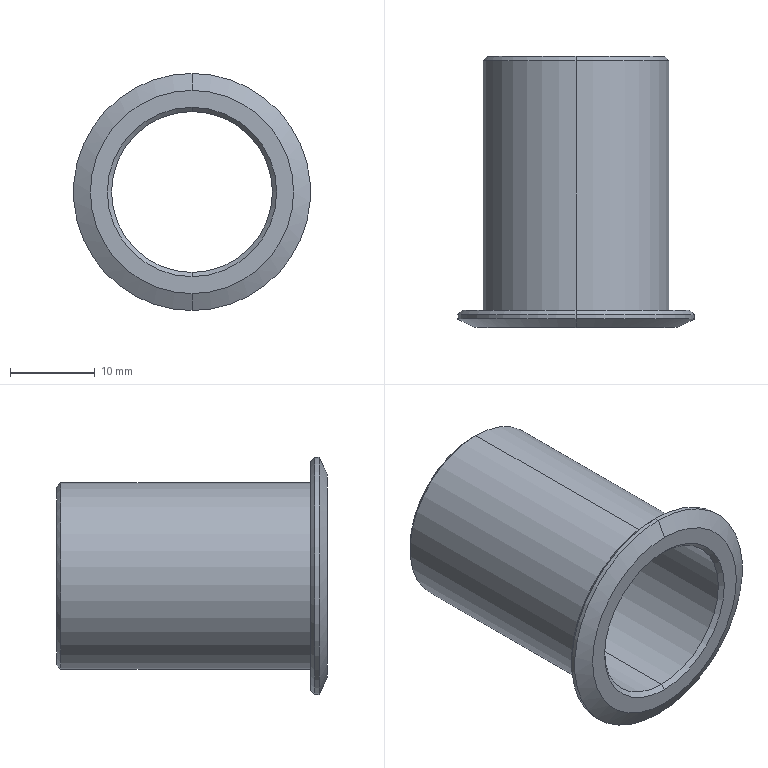Part | SolidWorks | features Chamfer 2, Revolution 1 | 1 solid | 19 faces | box 28 x 32 x 28 mm | volume 3444 mm3 | cone 10 | cylinder 6 | plane 3 | commonest cylinder face diameters 19 x2 22 x2 28 x2
STEP:
#1=CARTESIAN_POINT('',(0.,0.,-12.));
#2=VERTEX_POINT('',#1);
#3=CARTESIAN_POINT('',(0.,0.,12.));
#4=VERTEX_POINT('',#3);
#5=CARTESIAN_POINT('',(0.,0.,0.));
#6=DIRECTION('',(0.,-1.,0.));
#7=DIRECTION('',(0.,0.,-1.));
#8=AXIS2_PLACEMENT_3D('',#5,#6,#7);
#9=CIRCLE('',#8,12.);
#10=EDGE_CURVE('',#2,#4,#9,.T.);
#11=ORIENTED_EDGE('',*,*,#10,.F.);
#12=CARTESIAN_POINT('',(0.,1.,-14.));
#13=VERTEX_POINT('',#12);
#14=CARTESIAN_POINT('',(0.,0.,-12.));
#15=DIRECTION('',(0.,0.4472,-0.8944));
#16=VECTOR('',#15,1000.);
#17=LINE('',#14,#16);
#18=EDGE_CURVE('',#2,#13,#17,.T.);
#19=ORIENTED_EDGE('',*,*,#18,.T.);
#20=CARTESIAN_POINT('',(0.,1.,14.));
#21=VERTEX_POINT('',#20);
#22=CARTESIAN_POINT('',(0.,1.,0.));
#23=DIRECTION('',(0.,1.,0.));
#24=DIRECTION('',(0.,0.,-1.));
#25=AXIS2_PLACEMENT_3D('',#22,#23,#24);
#26=CIRCLE('',#25,14.);
#27=EDGE_CURVE('',#21,#13,#26,.T.);
#28=ORIENTED_EDGE('',*,*,#27,.F.);
#29=CARTESIAN_POINT('',(0.,0.,12.));
#30=DIRECTION('',(0.,0.4472,0.8944));
#31=VECTOR('',#30,1000.);
#32=LINE('',#29,#31);
#33=EDGE_CURVE('',#4,#21,#32,.T.);
#34=ORIENTED_EDGE('',*,*,#33,.F.);
#35=EDGE_LOOP('',(#11,#19,#28,#34));
#36=FACE_OUTER_BOUND('',#35,.T.);
#37=CARTESIAN_POINT('',(0.,0.,0.));
#38=DIRECTION('',(0.,1.,0.));
#39=DIRECTION('',(0.,0.,1.));
#40=AXIS2_PLACEMENT_3D('',#37,#38,#39);
#41=CONICAL_SURFACE('',#40,12.,1.107);
#42=ADVANCED_FACE('',(#36),#41,.T.);
#43=CARTESIAN_POINT('',(0.,0.5,9.5));
#44=VERTEX_POINT('',#43);
#45=CARTESIAN_POINT('',(0.,0.5,-9.5));
#46=VERTEX_POINT('',#45);
#47=CARTESIAN_POINT('',(0.,0.5,0.));
#48=DIRECTION('',(0.,-1.,0.));
#49=DIRECTION('',(0.,0.,-1.));
#50=AXIS2_PLACEMENT_3D('',#47,#48,#49);
#51=CIRCLE('',#50,9.5);
#52=EDGE_CURVE('',#44,#46,#51,.T.);
#53=ORIENTED_EDGE('',*,*,#52,.F.);
#54=CARTESIAN_POINT('',(0.,0.,10.));
#55=VERTEX_POINT('',#54);
#56=CARTESIAN_POINT('',(0.,0.5,9.5));
#57=DIRECTION('',(0.,-0.7071,0.7071));
#58=VECTOR('',#57,1000.);
#59=LINE('',#56,#58);
#60=EDGE_CURVE('',#44,#55,#59,.T.);
#61=ORIENTED_EDGE('',*,*,#60,.T.);
#62=CARTESIAN_POINT('',(0.,0.,-10.));
#63=VERTEX_POINT('',#62);
#64=CARTESIAN_POINT('',(0.,0.,0.));
#65=DIRECTION('',(0.,1.,0.));
#66=DIRECTION('',(0.,0.,-1.));
#67=AXIS2_PLACEMENT_3D('',#64,#65,#66);
#68=CIRCLE('',#67,10.);
#69=EDGE_CURVE('',#63,#55,#68,.T.);
#70=ORIENTED_EDGE('',*,*,#69,.F.);
#71=CARTESIAN_POINT('',(0.,0.5,-9.5));
#72=DIRECTION('',(0.,-0.7071,-0.7071));
#73=VECTOR('',#72,1000.);
#74=LINE('',#71,#73);
#75=EDGE_CURVE('',#46,#63,#74,.T.);
#76=ORIENTED_EDGE('',*,*,#75,.F.);
#77=EDGE_LOOP('',(#53,#61,#70,#76));
#78=FACE_OUTER_BOUND('',#77,.T.);
#79=CARTESIAN_POINT('',(0.,0.5,0.));
#80=DIRECTION('',(0.,-1.,0.));
#81=DIRECTION('',(0.,0.,-1.));
#82=AXIS2_PLACEMENT_3D('',#79,#80,#81);
#83=CONICAL_SURFACE('',#82,9.5,0.7854);
#84=ADVANCED_FACE('',(#78),#83,.F.);
#85=CARTESIAN_POINT('',(0.,31.5,-9.5));
#86=VERTEX_POINT('',#85);
#87=CARTESIAN_POINT('',(0.,31.5,9.5));
#88=VERTEX_POINT('',#87);
#89=CARTESIAN_POINT('',(0.,31.5,0.));
#90=DIRECTION('',(0.,1.,0.));
#91=DIRECTION('',(0.,0.,1.));
#92=AXIS2_PLACEMENT_3D('',#89,#90,#91);
#93=CIRCLE('',#92,9.5);
#94=EDGE_CURVE('',#86,#88,#93,.T.);
#95=ORIENTED_EDGE('',*,*,#94,.F.);
#96=CARTESIAN_POINT('',(0.,32.,-10.));
#97=VERTEX_POINT('',#96);
#98=CARTESIAN_POINT('',(0.,32.,-10.));
#99=DIRECTION('',(0.,0.7071,-0.7071));
#100=VECTOR('',#99,1000.);
#101=LINE('',#98,#100);
#102=EDGE_CURVE('',#86,#97,#101,.T.);
#103=ORIENTED_EDGE('',*,*,#102,.T.);
#104=CARTESIAN_POINT('',(0.,32.,10.));
#105=VERTEX_POINT('',#104);
#106=CARTESIAN_POINT('',(0.,32.,0.));
#107=DIRECTION('',(0.,-1.,0.));
#108=DIRECTION('',(0.,0.,1.));
#109=AXIS2_PLACEMENT_3D('',#106,#107,#108);
#110=CIRCLE('',#109,10.);
#111=EDGE_CURVE('',#105,#97,#110,.T.);
#112=ORIENTED_EDGE('',*,*,#111,.F.);
#113=CARTESIAN_POINT('',(0.,32.,10.));
#114=DIRECTION('',(0.,0.7071,0.7071));
#115=VECTOR('',#114,1000.);
#116=LINE('',#113,#115);
#117=EDGE_CURVE('',#88,#105,#116,.T.);
#118=ORIENTED_EDGE('',*,*,#117,.F.);
#119=EDGE_LOOP('',(#95,#103,#112,#118));
#120=FACE_OUTER_BOUND('',#119,.T.);
#121=CARTESIAN_POINT('',(0.,32.,0.));
#122=DIRECTION('',(0.,1.,0.));
#123=DIRECTION('',(0.,0.,1.));
#124=AXIS2_PLACEMENT_3D('',#121,#122,#123);
#125=CONICAL_SURFACE('',#124,10.,0.7854);
#126=ADVANCED_FACE('',(#120),#125,.F.);
#127=CARTESIAN_POINT('',(0.,32.,10.5));
#128=VERTEX_POINT('',#127);
#129=CARTESIAN_POINT('',(0.,32.,-10.5));
#130=VERTEX_POINT('',#129);
#131=CARTESIAN_POINT('',(0.,32.,0.));
#132=DIRECTION('',(0.,1.,0.));
#133=DIRECTION('',(0.,0.,1.));
#134=AXIS2_PLACEMENT_3D('',#131,#132,#133);
#135=CIRCLE('',#134,10.5);
#136=EDGE_CURVE('',#128,#130,#135,.T.);
#137=ORIENTED_EDGE('',*,*,#136,.F.);
#138=CARTESIAN_POINT('',(0.,31.5,11.));
#139=VERTEX_POINT('',#138);
#140=CARTESIAN_POINT('',(0.,31.5,11.));
#141=DIRECTION('',(0.,-0.7071,0.7071));
#142=VECTOR('',#141,1000.);
#143=LINE('',#140,#142);
#144=EDGE_CURVE('',#128,#139,#143,.T.);
#145=ORIENTED_EDGE('',*,*,#144,.T.);
#146=CARTESIAN_POINT('',(0.,31.5,-11.));
#147=VERTEX_POINT('',#146);
#148=CARTESIAN_POINT('',(0.,31.5,0.));
#149=DIRECTION('',(0.,-1.,0.));
#150=DIRECTION('',(0.,0.,1.));
#151=AXIS2_PLACEMENT_3D('',#148,#149,#150);
#152=CIRCLE('',#151,11.);
#153=EDGE_CURVE('',#147,#139,#152,.T.);
#154=ORIENTED_EDGE('',*,*,#153,.F.);
#155=CARTESIAN_POINT('',(0.,31.5,-11.));
#156=DIRECTION('',(0.,-0.7071,-0.7071));
#157=VECTOR('',#156,1000.);
#158=LINE('',#155,#157);
#159=EDGE_CURVE('',#130,#147,#158,.T.);
#160=ORIENTED_EDGE('',*,*,#159,.F.);
#161=EDGE_LOOP('',(#137,#145,#154,#160));
#162=FACE_OUTER_BOUND('',#161,.T.);
#163=CARTESIAN_POINT('',(0.,31.5,0.));
#164=DIRECTION('',(0.,-1.,0.));
#165=DIRECTION('',(0.,0.,-1.));
#166=AXIS2_PLACEMENT_3D('',#163,#164,#165);
#167=CONICAL_SURFACE('',#166,11.,0.7854);
#168=ADVANCED_FACE('',(#162),#167,.T.);
#169=CARTESIAN_POINT('',(0.,2.,13.5));
#170=VERTEX_POINT('',#169);
#171=CARTESIAN_POINT('',(0.,2.,-13.5));
#172=VERTEX_POINT('',#171);
#173=CARTESIAN_POINT('',(0.,2.,0.));
#174=DIRECTION('',(0.,1.,0.));
#175=DIRECTION('',(0.,0.,1.));
#176=AXIS2_PLACEMENT_3D('',#173,#174,#175);
#177=CIRCLE('',#176,13.5);
#178=EDGE_CURVE('',#170,#172,#177,.T.);
#179=ORIENTED_EDGE('',*,*,#178,.F.);
#180=CARTESIAN_POINT('',(0.,1.5,14.));
#181=VERTEX_POINT('',#180);
#182=CARTESIAN_POINT('',(0.,1.5,14.));
#183=DIRECTION('',(0.,-0.7071,0.7071));
#184=VECTOR('',#183,1000.);
#185=LINE('',#182,#184);
#186=EDGE_CURVE('',#170,#181,#185,.T.);
#187=ORIENTED_EDGE('',*,*,#186,.T.);
#188=CARTESIAN_POINT('',(0.,1.5,-14.));
#189=VERTEX_POINT('',#188);
#190=CARTESIAN_POINT('',(0.,1.5,0.));
#191=DIRECTION('',(0.,-1.,0.));
#192=DIRECTION('',(0.,0.,1.));
#193=AXIS2_PLACEMENT_3D('',#190,#191,#192);
#194=CIRCLE('',#193,14.);
#195=EDGE_CURVE('',#189,#181,#194,.T.);
#196=ORIENTED_EDGE('',*,*,#195,.F.);
#197=CARTESIAN_POINT('',(0.,1.5,-14.));
#198=DIRECTION('',(0.,-0.7071,-0.7071));
#199=VECTOR('',#198,1000.);
#200=LINE('',#197,#199);
#201=EDGE_CURVE('',#172,#189,#200,.T.);
#202=ORIENTED_EDGE('',*,*,#201,.F.);
#203=EDGE_LOOP('',(#179,#187,#196,#202));
#204=FACE_OUTER_BOUND('',#203,.T.);
#205=CARTESIAN_POINT('',(0.,1.5,0.));
#206=DIRECTION('',(0.,-1.,0.));
#207=DIRECTION('',(0.,0.,-1.));
#208=AXIS2_PLACEMENT_3D('',#205,#206,#207);
#209=CONICAL_SURFACE('',#208,14.,0.7854);
#210=ADVANCED_FACE('',(#204),#209,.T.);
#211=ORIENTED_EDGE('',*,*,#153,.T.);
#212=CARTESIAN_POINT('',(0.,2.,11.));
#213=VERTEX_POINT('',#212);
#214=CARTESIAN_POINT('',(0.,0.,11.));
#215=DIRECTION('',(0.,-1.,0.));
#216=VECTOR('',#215,1000.);
#217=LINE('',#214,#216);
#218=EDGE_CURVE('',#139,#213,#217,.T.);
#219=ORIENTED_EDGE('',*,*,#218,.T.);
#220=CARTESIAN_POINT('',(0.,2.,-11.));
#221=VERTEX_POINT('',#220);
#222=CARTESIAN_POINT('',(0.,2.,0.));
#223=DIRECTION('',(0.,-1.,0.));
#224=DIRECTION('',(0.,0.,-1.));
#225=AXIS2_PLACEMENT_3D('',#222,#223,#224);
#226=CIRCLE('',#225,11.);
#227=EDGE_CURVE('',#221,#213,#226,.T.);
#228=ORIENTED_EDGE('',*,*,#227,.F.);
#229=CARTESIAN_POINT('',(0.,0.,-11.));
#230=DIRECTION('',(0.,-1.,0.));
#231=VECTOR('',#230,1000.);
#232=LINE('',#229,#231);
#233=EDGE_CURVE('',#147,#221,#232,.T.);
#234=ORIENTED_EDGE('',*,*,#233,.F.);
#235=EDGE_LOOP('',(#211,#219,#228,#234));
#236=FACE_OUTER_BOUND('',#235,.T.);
#237=CARTESIAN_POINT('',(0.,0.,0.));
#238=DIRECTION('',(0.,-1.,0.));
#239=DIRECTION('',(0.,0.,-1.));
#240=AXIS2_PLACEMENT_3D('',#237,#238,#239);
#241=CYLINDRICAL_SURFACE('',#240,11.);
#242=ADVANCED_FACE('',(#236),#241,.T.);
#243=ORIENTED_EDGE('',*,*,#195,.T.);
#244=CARTESIAN_POINT('',(0.,0.,14.));
#245=DIRECTION('',(0.,-1.,0.));
#246=VECTOR('',#245,1000.);
#247=LINE('',#244,#246);
#248=EDGE_CURVE('',#181,#21,#247,.T.);
#249=ORIENTED_EDGE('',*,*,#248,.T.);
#250=ORIENTED_EDGE('',*,*,#27,.T.);
#251=CARTESIAN_POINT('',(0.,0.,-14.));
#252=DIRECTION('',(0.,-1.,0.));
#253=VECTOR('',#252,1000.);
#254=LINE('',#251,#253);
#255=EDGE_CURVE('',#189,#13,#254,.T.);
#256=ORIENTED_EDGE('',*,*,#255,.F.);
#257=EDGE_LOOP('',(#243,#249,#250,#256));
#258=FACE_OUTER_BOUND('',#257,.T.);
#259=CARTESIAN_POINT('',(0.,0.,0.));
#260=DIRECTION('',(0.,-1.,0.));
#261=DIRECTION('',(0.,0.,-1.));
#262=AXIS2_PLACEMENT_3D('',#259,#260,#261);
#263=CYLINDRICAL_SURFACE('',#262,14.);
#264=ADVANCED_FACE('',(#258),#263,.T.);
#265=ORIENTED_EDGE('',*,*,#94,.T.);
#266=CARTESIAN_POINT('',(0.,0.,9.5));
#267=DIRECTION('',(0.,-1.,0.));
#268=VECTOR('',#267,1000.);
#269=LINE('',#266,#268);
#270=EDGE_CURVE('',#88,#44,#269,.T.);
#271=ORIENTED_EDGE('',*,*,#270,.T.);
#272=ORIENTED_EDGE('',*,*,#52,.T.);
#273=CARTESIAN_POINT('',(0.,0.,-9.5));
#274=DIRECTION('',(0.,-1.,0.));
#275=VECTOR('',#274,1000.);
#276=LINE('',#273,#275);
#277=EDGE_CURVE('',#86,#46,#276,.T.);
#278=ORIENTED_EDGE('',*,*,#277,.F.);
#279=EDGE_LOOP('',(#265,#271,#272,#278));
#280=FACE_OUTER_BOUND('',#279,.T.);
#281=CARTESIAN_POINT('',(0.,0.,0.));
#282=DIRECTION('',(0.,-1.,0.));
#283=DIRECTION('',(0.,0.,-1.));
#284=AXIS2_PLACEMENT_3D('',#281,#282,#283);
#285=CYLINDRICAL_SURFACE('',#284,9.5);
#286=ADVANCED_FACE('',(#280),#285,.F.);
#287=ORIENTED_EDGE('',*,*,#270,.F.);
#288=CARTESIAN_POINT('',(0.,31.5,0.));
#289=DIRECTION('',(0.,1.,0.));
#290=DIRECTION('',(0.,0.,1.));
#291=AXIS2_PLACEMENT_3D('',#288,#289,#290);
#292=CIRCLE('',#291,9.5);
#293=EDGE_CURVE('',#88,#86,#292,.T.);
#294=ORIENTED_EDGE('',*,*,#293,.T.);
#295=ORIENTED_EDGE('',*,*,#277,.T.);
#296=CARTESIAN_POINT('',(0.,0.5,0.));
#297=DIRECTION('',(0.,-1.,0.));
#298=DIRECTION('',(0.,0.,-1.));
#299=AXIS2_PLACEMENT_3D('',#296,#297,#298);
#300=CIRCLE('',#299,9.5);
#301=EDGE_CURVE('',#46,#44,#300,.T.);
#302=ORIENTED_EDGE('',*,*,#301,.T.);
#303=EDGE_LOOP('',(#287,#294,#295,#302));
#304=FACE_OUTER_BOUND('',#303,.T.);
#305=CARTESIAN_POINT('',(0.,0.,0.));
#306=DIRECTION('',(0.,-1.,0.));
#307=DIRECTION('',(0.,0.,-1.));
#308=AXIS2_PLACEMENT_3D('',#305,#306,#307);
#309=CYLINDRICAL_SURFACE('',#308,9.5);
#310=ADVANCED_FACE('',(#304),#309,.F.);
#311=CARTESIAN_POINT('',(0.,0.,0.));
#312=DIRECTION('',(0.,-1.,0.));
#313=DIRECTION('',(0.,0.,-1.));
#314=AXIS2_PLACEMENT_3D('',#311,#312,#313);
#315=CIRCLE('',#314,12.);
#316=EDGE_CURVE('',#4,#2,#315,.T.);
#317=ORIENTED_EDGE('',*,*,#316,.T.);
#318=ORIENTED_EDGE('',*,*,#10,.T.);
#319=EDGE_LOOP('',(#317,#318));
#320=FACE_OUTER_BOUND('',#319,.T.);
#321=ORIENTED_EDGE('',*,*,#69,.T.);
#322=CARTESIAN_POINT('',(0.,0.,0.));
#323=DIRECTION('',(0.,1.,0.));
#324=DIRECTION('',(0.,0.,-1.));
#325=AXIS2_PLACEMENT_3D('',#322,#323,#324);
#326=CIRCLE('',#325,10.);
#327=EDGE_CURVE('',#55,#63,#326,.T.);
#328=ORIENTED_EDGE('',*,*,#327,.T.);
#329=EDGE_LOOP('',(#321,#328));
#330=FACE_BOUND('',#329,.T.);
#331=CARTESIAN_POINT('',(9.5,0.,0.));
#332=DIRECTION('',(0.,-1.,0.));
#333=DIRECTION('',(0.,0.,-1.));
#334=AXIS2_PLACEMENT_3D('',#331,#332,#333);
#335=PLANE('',#334);
#336=ADVANCED_FACE('',(#320,#330),#335,.T.);
#337=ORIENTED_EDGE('',*,*,#248,.F.);
#338=CARTESIAN_POINT('',(0.,1.5,0.));
#339=DIRECTION('',(0.,-1.,0.));
#340=DIRECTION('',(0.,0.,1.));
#341=AXIS2_PLACEMENT_3D('',#338,#339,#340);
#342=CIRCLE('',#341,14.);
#343=EDGE_CURVE('',#181,#189,#342,.T.);
#344=ORIENTED_EDGE('',*,*,#343,.T.);
#345=ORIENTED_EDGE('',*,*,#255,.T.);
#346=CARTESIAN_POINT('',(0.,1.,0.));
#347=DIRECTION('',(0.,1.,0.));
#348=DIRECTION('',(0.,0.,-1.));
#349=AXIS2_PLACEMENT_3D('',#346,#347,#348);
#350=CIRCLE('',#349,14.);
#351=EDGE_CURVE('',#13,#21,#350,.T.);
#352=ORIENTED_EDGE('',*,*,#351,.T.);
#353=EDGE_LOOP('',(#337,#344,#345,#352));
#354=FACE_OUTER_BOUND('',#353,.T.);
#355=CARTESIAN_POINT('',(0.,0.,0.));
#356=DIRECTION('',(0.,-1.,0.));
#357=DIRECTION('',(0.,0.,-1.));
#358=AXIS2_PLACEMENT_3D('',#355,#356,#357);
#359=CYLINDRICAL_SURFACE('',#358,14.);
#360=ADVANCED_FACE('',(#354),#359,.T.);
#361=CARTESIAN_POINT('',(0.,2.,0.));
#362=DIRECTION('',(0.,1.,0.));
#363=DIRECTION('',(0.,0.,1.));
#364=AXIS2_PLACEMENT_3D('',#361,#362,#363);
#365=CIRCLE('',#364,13.5);
#366=EDGE_CURVE('',#172,#170,#365,.T.);
#367=ORIENTED_EDGE('',*,*,#366,.T.);
#368=ORIENTED_EDGE('',*,*,#178,.T.);
#369=EDGE_LOOP('',(#367,#368));
#370=FACE_OUTER_BOUND('',#369,.T.);
#371=ORIENTED_EDGE('',*,*,#227,.T.);
#372=CARTESIAN_POINT('',(0.,2.,0.));
#373=DIRECTION('',(0.,-1.,0.));
#374=DIRECTION('',(0.,0.,-1.));
#375=AXIS2_PLACEMENT_3D('',#372,#373,#374);
#376=CIRCLE('',#375,11.);
#377=EDGE_CURVE('',#213,#221,#376,.T.);
#378=ORIENTED_EDGE('',*,*,#377,.T.);
#379=EDGE_LOOP('',(#371,#378));
#380=FACE_BOUND('',#379,.T.);
#381=CARTESIAN_POINT('',(14.,2.,0.));
#382=DIRECTION('',(0.,1.,0.));
#383=DIRECTION('',(0.,0.,1.));
#384=AXIS2_PLACEMENT_3D('',#381,#382,#383);
#385=PLANE('',#384);
#386=ADVANCED_FACE('',(#370,#380),#385,.T.);
#387=ORIENTED_EDGE('',*,*,#218,.F.);
#388=CARTESIAN_POINT('',(0.,31.5,0.));
#389=DIRECTION('',(0.,-1.,0.));
#390=DIRECTION('',(0.,0.,1.));
#391=AXIS2_PLACEMENT_3D('',#388,#389,#390);
#392=CIRCLE('',#391,11.);
#393=EDGE_CURVE('',#139,#147,#392,.T.);
#394=ORIENTED_EDGE('',*,*,#393,.T.);
#395=ORIENTED_EDGE('',*,*,#233,.T.);
#396=ORIENTED_EDGE('',*,*,#377,.F.);
#397=EDGE_LOOP('',(#387,#394,#395,#396));
#398=FACE_OUTER_BOUND('',#397,.T.);
#399=CARTESIAN_POINT('',(0.,0.,0.));
#400=DIRECTION('',(0.,-1.,0.));
#401=DIRECTION('',(0.,0.,-1.));
#402=AXIS2_PLACEMENT_3D('',#399,#400,#401);
#403=CYLINDRICAL_SURFACE('',#402,11.);
#404=ADVANCED_FACE('',(#398),#403,.T.);
#405=CARTESIAN_POINT('',(0.,32.,0.));
#406=DIRECTION('',(0.,1.,0.));
#407=DIRECTION('',(0.,0.,1.));
#408=AXIS2_PLACEMENT_3D('',#405,#406,#407);
#409=CIRCLE('',#408,10.5);
#410=EDGE_CURVE('',#130,#128,#409,.T.);
#411=ORIENTED_EDGE('',*,*,#410,.T.);
#412=ORIENTED_EDGE('',*,*,#136,.T.);
#413=EDGE_LOOP('',(#411,#412));
#414=FACE_OUTER_BOUND('',#413,.T.);
#415=ORIENTED_EDGE('',*,*,#111,.T.);
#416=CARTESIAN_POINT('',(0.,32.,0.));
#417=DIRECTION('',(0.,-1.,0.));
#418=DIRECTION('',(0.,0.,1.));
#419=AXIS2_PLACEMENT_3D('',#416,#417,#418);
#420=CIRCLE('',#419,10.);
#421=EDGE_CURVE('',#97,#105,#420,.T.);
#422=ORIENTED_EDGE('',*,*,#421,.T.);
#423=EDGE_LOOP('',(#415,#422));
#424=FACE_BOUND('',#423,.T.);
#425=CARTESIAN_POINT('',(11.,32.,0.));
#426=DIRECTION('',(0.,1.,0.));
#427=DIRECTION('',(0.,0.,1.));
#428=AXIS2_PLACEMENT_3D('',#425,#426,#427);
#429=PLANE('',#428);
#430=ADVANCED_FACE('',(#414,#424),#429,.T.);
#431=ORIENTED_EDGE('',*,*,#186,.F.);
#432=ORIENTED_EDGE('',*,*,#366,.F.);
#433=ORIENTED_EDGE('',*,*,#201,.T.);
#434=ORIENTED_EDGE('',*,*,#343,.F.);
#435=EDGE_LOOP('',(#431,#432,#433,#434));
#436=FACE_OUTER_BOUND('',#435,.T.);
#437=CARTESIAN_POINT('',(0.,1.5,0.));
#438=DIRECTION('',(0.,-1.,0.));
#439=DIRECTION('',(0.,0.,-1.));
#440=AXIS2_PLACEMENT_3D('',#437,#438,#439);
#441=CONICAL_SURFACE('',#440,14.,0.7854);
#442=ADVANCED_FACE('',(#436),#441,.T.);
#443=ORIENTED_EDGE('',*,*,#144,.F.);
#444=ORIENTED_EDGE('',*,*,#410,.F.);
#445=ORIENTED_EDGE('',*,*,#159,.T.);
#446=ORIENTED_EDGE('',*,*,#393,.F.);
#447=EDGE_LOOP('',(#443,#444,#445,#446));
#448=FACE_OUTER_BOUND('',#447,.T.);
#449=CARTESIAN_POINT('',(0.,31.5,0.));
#450=DIRECTION('',(0.,-1.,0.));
#451=DIRECTION('',(0.,0.,-1.));
#452=AXIS2_PLACEMENT_3D('',#449,#450,#451);
#453=CONICAL_SURFACE('',#452,11.,0.7854);
#454=ADVANCED_FACE('',(#448),#453,.T.);
#455=ORIENTED_EDGE('',*,*,#102,.F.);
#456=ORIENTED_EDGE('',*,*,#293,.F.);
#457=ORIENTED_EDGE('',*,*,#117,.T.);
#458=ORIENTED_EDGE('',*,*,#421,.F.);
#459=EDGE_LOOP('',(#455,#456,#457,#458));
#460=FACE_OUTER_BOUND('',#459,.T.);
#461=CARTESIAN_POINT('',(0.,32.,0.));
#462=DIRECTION('',(0.,1.,0.));
#463=DIRECTION('',(0.,0.,1.));
#464=AXIS2_PLACEMENT_3D('',#461,#462,#463);
#465=CONICAL_SURFACE('',#464,10.,0.7854);
#466=ADVANCED_FACE('',(#460),#465,.F.);
#467=ORIENTED_EDGE('',*,*,#60,.F.);
#468=ORIENTED_EDGE('',*,*,#301,.F.);
#469=ORIENTED_EDGE('',*,*,#75,.T.);
#470=ORIENTED_EDGE('',*,*,#327,.F.);
#471=EDGE_LOOP('',(#467,#468,#469,#470));
#472=FACE_OUTER_BOUND('',#471,.T.);
#473=CARTESIAN_POINT('',(0.,0.5,0.));
#474=DIRECTION('',(0.,-1.,0.));
#475=DIRECTION('',(0.,0.,-1.));
#476=AXIS2_PLACEMENT_3D('',#473,#474,#475);
#477=CONICAL_SURFACE('',#476,9.5,0.7854);
#478=ADVANCED_FACE('',(#472),#477,.F.);
#479=ORIENTED_EDGE('',*,*,#18,.F.);
#480=ORIENTED_EDGE('',*,*,#316,.F.);
#481=ORIENTED_EDGE('',*,*,#33,.T.);
#482=ORIENTED_EDGE('',*,*,#351,.F.);
#483=EDGE_LOOP('',(#479,#480,#481,#482));
#484=FACE_OUTER_BOUND('',#483,.T.);
#485=CARTESIAN_POINT('',(0.,0.,0.));
#486=DIRECTION('',(0.,1.,0.));
#487=DIRECTION('',(0.,0.,1.));
#488=AXIS2_PLACEMENT_3D('',#485,#486,#487);
#489=CONICAL_SURFACE('',#488,12.,1.107);
#490=ADVANCED_FACE('',(#484),#489,.T.);
#491=CLOSED_SHELL('',(#42,#84,#126,#168,#210,#242,#264,#286,#310,#336,#360,#386,#404,#430,#442,#454,#466,#478,#490));
#492=MANIFOLD_SOLID_BREP('',#491);
#493=CARTESIAN_POINT('',(0.,0.,0.));
#494=DIRECTION('',(0.,0.,1.));
#495=DIRECTION('',(1.,0.,0.));
#496=AXIS2_PLACEMENT_3D('',#493,#494,#495);
#497=(LENGTH_UNIT()NAMED_UNIT(*)SI_UNIT(.MILLI.,.METRE.));
#498=UNCERTAINTY_MEASURE_WITH_UNIT(LENGTH_MEASURE(0.00001),#497,'','');
#499=(NAMED_UNIT(*)PLANE_ANGLE_UNIT()SI_UNIT($,.RADIAN.));
#500=(NAMED_UNIT(*)SI_UNIT($,.STERADIAN.)SOLID_ANGLE_UNIT());
#501=(GEOMETRIC_REPRESENTATION_CONTEXT(3)GLOBAL_UNCERTAINTY_ASSIGNED_CONTEXT((#498))GLOBAL_UNIT_ASSIGNED_CONTEXT((#497,#499,#500))REPRESENTATION_CONTEXT('',''));
#502=ADVANCED_BREP_SHAPE_REPRESENTATION('',(#492,#496),#501);